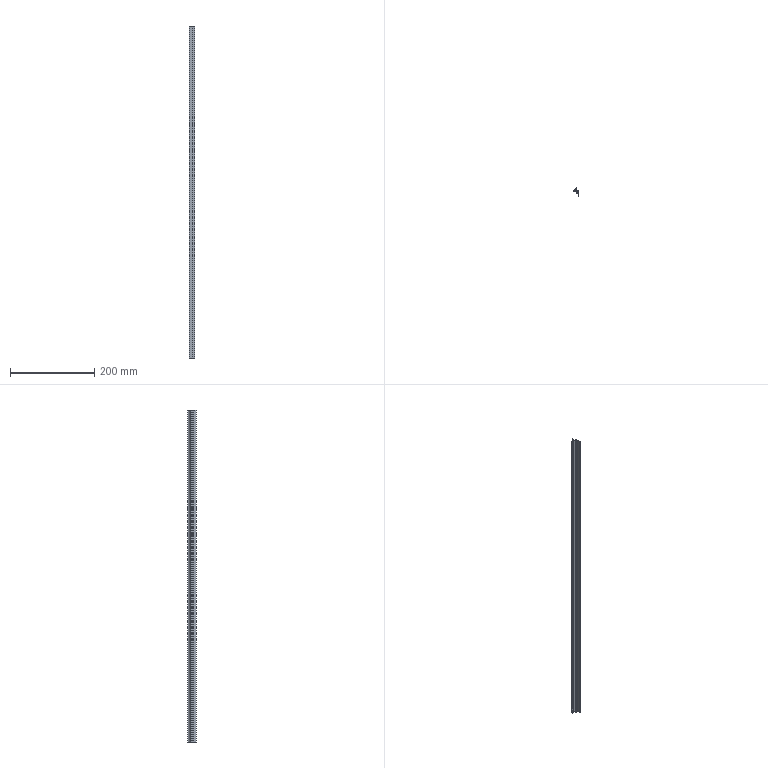Part | SolidWorks | features BaseBody 1, ICE 1, MoveFace 1 | 1 solid | 27 faces | box 14 x 20.3 x 788 mm | volume 40122 mm3 | plane 20 | cylinder 7 | commonest cylinder face diameters 0.387 x2 0.8 x2 0.4 x1 20 x1 22 x1
STEP:
#1=CARTESIAN_POINT('',(-5.304,-0.625,200.));
#2=VERTEX_POINT('',#1);
#3=CARTESIAN_POINT('',(-5.449,-0.8125,200.));
#4=VERTEX_POINT('',#3);
#5=CARTESIAN_POINT('',(-5.255,-0.8125,200.));
#6=DIRECTION('',(0.,0.,1.));
#7=DIRECTION('',(-1.,0.,0.));
#8=AXIS2_PLACEMENT_3D('',#5,#6,#7);
#9=CIRCLE('',#8,0.1937);
#10=EDGE_CURVE('',#2,#4,#9,.T.);
#11=ORIENTED_EDGE('',*,*,#10,.T.);
#12=CARTESIAN_POINT('',(-5.449,-0.8125,-588.));
#13=VERTEX_POINT('',#12);
#14=CARTESIAN_POINT('',(-5.449,-0.8125,230.));
#15=DIRECTION('',(0.,0.,-1.));
#16=VECTOR('',#15,1000.);
#17=LINE('',#14,#16);
#18=EDGE_CURVE('',#4,#13,#17,.T.);
#19=ORIENTED_EDGE('',*,*,#18,.T.);
#20=CARTESIAN_POINT('',(-5.304,-0.625,-588.));
#21=VERTEX_POINT('',#20);
#22=CARTESIAN_POINT('',(-5.255,-0.8125,-588.));
#23=DIRECTION('',(0.,0.,-1.));
#24=DIRECTION('',(1.,0.,0.));
#25=AXIS2_PLACEMENT_3D('',#22,#23,#24);
#26=CIRCLE('',#25,0.1937);
#27=EDGE_CURVE('',#13,#21,#26,.T.);
#28=ORIENTED_EDGE('',*,*,#27,.T.);
#29=CARTESIAN_POINT('',(-5.304,-0.625,230.));
#30=DIRECTION('',(0.,0.,-1.));
#31=VECTOR('',#30,1000.);
#32=LINE('',#29,#31);
#33=EDGE_CURVE('',#2,#21,#32,.T.);
#34=ORIENTED_EDGE('',*,*,#33,.F.);
#35=EDGE_LOOP('',(#11,#19,#28,#34));
#36=FACE_OUTER_BOUND('',#35,.T.);
#37=CARTESIAN_POINT('',(-5.255,-0.8125,230.));
#38=DIRECTION('',(0.,0.,-1.));
#39=DIRECTION('',(-1.,0.,0.));
#40=AXIS2_PLACEMENT_3D('',#37,#38,#39);
#41=CYLINDRICAL_SURFACE('',#40,0.1937);
#42=ADVANCED_FACE('',(#36),#41,.F.);
#43=CARTESIAN_POINT('',(5.,-1.,-588.));
#44=VERTEX_POINT('',#43);
#45=CARTESIAN_POINT('',(5.,-14.3,-588.));
#46=VERTEX_POINT('',#45);
#47=CARTESIAN_POINT('',(5.,29.623,-588.));
#48=DIRECTION('',(0.,-1.,0.));
#49=VECTOR('',#48,1000.);
#50=LINE('',#47,#49);
#51=EDGE_CURVE('',#44,#46,#50,.T.);
#52=ORIENTED_EDGE('',*,*,#51,.F.);
#53=CARTESIAN_POINT('',(5.,-1.,200.));
#54=VERTEX_POINT('',#53);
#55=CARTESIAN_POINT('',(5.,-1.,230.));
#56=DIRECTION('',(0.,0.,-1.));
#57=VECTOR('',#56,1000.);
#58=LINE('',#55,#57);
#59=EDGE_CURVE('',#54,#44,#58,.T.);
#60=ORIENTED_EDGE('',*,*,#59,.F.);
#61=CARTESIAN_POINT('',(5.,-14.3,200.));
#62=VERTEX_POINT('',#61);
#63=CARTESIAN_POINT('',(5.,-14.3,200.));
#64=DIRECTION('',(0.,1.,0.));
#65=VECTOR('',#64,1000.);
#66=LINE('',#63,#65);
#67=EDGE_CURVE('',#62,#54,#66,.T.);
#68=ORIENTED_EDGE('',*,*,#67,.F.);
#69=CARTESIAN_POINT('',(5.,-14.3,230.));
#70=DIRECTION('',(0.,0.,1.));
#71=VECTOR('',#70,1000.);
#72=LINE('',#69,#71);
#73=EDGE_CURVE('',#46,#62,#72,.T.);
#74=ORIENTED_EDGE('',*,*,#73,.F.);
#75=EDGE_LOOP('',(#52,#60,#68,#74));
#76=FACE_OUTER_BOUND('',#75,.T.);
#77=CARTESIAN_POINT('',(5.,-14.3,230.));
#78=DIRECTION('',(-1.,0.,0.));
#79=DIRECTION('',(0.,0.,1.));
#80=AXIS2_PLACEMENT_3D('',#77,#78,#79);
#81=PLANE('',#80);
#82=ADVANCED_FACE('',(#76),#81,.F.);
#83=CARTESIAN_POINT('',(-9.,-2.,-588.));
#84=VERTEX_POINT('',#83);
#85=CARTESIAN_POINT('',(-9.,-2.,200.));
#86=VERTEX_POINT('',#85);
#87=CARTESIAN_POINT('',(-9.,-2.,230.));
#88=DIRECTION('',(0.,0.,1.));
#89=VECTOR('',#88,1000.);
#90=LINE('',#87,#89);
#91=EDGE_CURVE('',#84,#86,#90,.T.);
#92=ORIENTED_EDGE('',*,*,#91,.F.);
#93=CARTESIAN_POINT('',(0.9,-2.,-588.));
#94=VERTEX_POINT('',#93);
#95=CARTESIAN_POINT('',(5.,-2.,-588.));
#96=DIRECTION('',(-1.,0.,0.));
#97=VECTOR('',#96,1000.);
#98=LINE('',#95,#97);
#99=EDGE_CURVE('',#94,#84,#98,.T.);
#100=ORIENTED_EDGE('',*,*,#99,.F.);
#101=CARTESIAN_POINT('',(0.9,-2.,200.));
#102=VERTEX_POINT('',#101);
#103=CARTESIAN_POINT('',(0.9,-2.,230.));
#104=DIRECTION('',(0.,0.,-1.));
#105=VECTOR('',#104,1000.);
#106=LINE('',#103,#105);
#107=EDGE_CURVE('',#102,#94,#106,.T.);
#108=ORIENTED_EDGE('',*,*,#107,.F.);
#109=CARTESIAN_POINT('',(5.,-2.,200.));
#110=DIRECTION('',(1.,0.,0.));
#111=VECTOR('',#110,1000.);
#112=LINE('',#109,#111);
#113=EDGE_CURVE('',#86,#102,#112,.T.);
#114=ORIENTED_EDGE('',*,*,#113,.F.);
#115=EDGE_LOOP('',(#92,#100,#108,#114));
#116=FACE_OUTER_BOUND('',#115,.T.);
#117=CARTESIAN_POINT('',(-9.,-2.,230.));
#118=DIRECTION('',(0.,1.,0.));
#119=DIRECTION('',(0.,0.,1.));
#120=AXIS2_PLACEMENT_3D('',#117,#118,#119);
#121=PLANE('',#120);
#122=ADVANCED_FACE('',(#116),#121,.F.);
#123=CARTESIAN_POINT('',(4.,-6.,200.));
#124=VERTEX_POINT('',#123);
#125=CARTESIAN_POINT('',(4.,-3.,200.));
#126=VERTEX_POINT('',#125);
#127=CARTESIAN_POINT('',(4.,29.623,200.));
#128=DIRECTION('',(0.,1.,0.));
#129=VECTOR('',#128,1000.);
#130=LINE('',#127,#129);
#131=EDGE_CURVE('',#124,#126,#130,.T.);
#132=ORIENTED_EDGE('',*,*,#131,.F.);
#133=CARTESIAN_POINT('',(1.,-6.,200.));
#134=VERTEX_POINT('',#133);
#135=CARTESIAN_POINT('',(5.,-6.,200.));
#136=DIRECTION('',(1.,0.,0.));
#137=VECTOR('',#136,1000.);
#138=LINE('',#135,#137);
#139=EDGE_CURVE('',#134,#124,#138,.T.);
#140=ORIENTED_EDGE('',*,*,#139,.F.);
#141=CARTESIAN_POINT('',(1.,-6.7,200.));
#142=VERTEX_POINT('',#141);
#143=CARTESIAN_POINT('',(1.,-6.,200.));
#144=DIRECTION('',(0.,-1.,0.));
#145=VECTOR('',#144,1000.);
#146=LINE('',#143,#145);
#147=EDGE_CURVE('',#134,#142,#146,.T.);
#148=ORIENTED_EDGE('',*,*,#147,.T.);
#149=CARTESIAN_POINT('',(-1.7,-6.7,200.));
#150=VERTEX_POINT('',#149);
#151=CARTESIAN_POINT('',(5.,-6.7,200.));
#152=DIRECTION('',(1.,0.,0.));
#153=VECTOR('',#152,1000.);
#154=LINE('',#151,#153);
#155=EDGE_CURVE('',#150,#142,#154,.T.);
#156=ORIENTED_EDGE('',*,*,#155,.F.);
#157=CARTESIAN_POINT('',(-1.7,-7.7,200.));
#158=VERTEX_POINT('',#157);
#159=CARTESIAN_POINT('',(-1.7,-6.7,200.));
#160=DIRECTION('',(0.,-1.,0.));
#161=VECTOR('',#160,1000.);
#162=LINE('',#159,#161);
#163=EDGE_CURVE('',#150,#158,#162,.T.);
#164=ORIENTED_EDGE('',*,*,#163,.T.);
#165=CARTESIAN_POINT('',(4.,-7.7,200.));
#166=VERTEX_POINT('',#165);
#167=CARTESIAN_POINT('',(5.,-7.7,200.));
#168=DIRECTION('',(-1.,0.,0.));
#169=VECTOR('',#168,1000.);
#170=LINE('',#167,#169);
#171=EDGE_CURVE('',#166,#158,#170,.T.);
#172=ORIENTED_EDGE('',*,*,#171,.F.);
#173=CARTESIAN_POINT('',(4.,-14.3,200.));
#174=VERTEX_POINT('',#173);
#175=CARTESIAN_POINT('',(4.,29.623,200.));
#176=DIRECTION('',(0.,1.,0.));
#177=VECTOR('',#176,1000.);
#178=LINE('',#175,#177);
#179=EDGE_CURVE('',#174,#166,#178,.T.);
#180=ORIENTED_EDGE('',*,*,#179,.F.);
#181=CARTESIAN_POINT('',(5.,-14.3,200.));
#182=DIRECTION('',(-1.,0.,0.));
#183=VECTOR('',#182,1000.);
#184=LINE('',#181,#183);
#185=EDGE_CURVE('',#62,#174,#184,.T.);
#186=ORIENTED_EDGE('',*,*,#185,.F.);
#187=ORIENTED_EDGE('',*,*,#67,.T.);
#188=CARTESIAN_POINT('',(-5.207,-1.,200.));
#189=VERTEX_POINT('',#188);
#190=CARTESIAN_POINT('',(5.,-1.,200.));
#191=DIRECTION('',(1.,0.,0.));
#192=VECTOR('',#191,1000.);
#193=LINE('',#190,#192);
#194=EDGE_CURVE('',#189,#54,#193,.T.);
#195=ORIENTED_EDGE('',*,*,#194,.F.);
#196=CARTESIAN_POINT('',(-5.255,-0.8125,200.));
#197=DIRECTION('',(0.,0.,1.));
#198=DIRECTION('',(-1.,0.,0.));
#199=AXIS2_PLACEMENT_3D('',#196,#197,#198);
#200=CIRCLE('',#199,0.1937);
#201=EDGE_CURVE('',#4,#189,#200,.T.);
#202=ORIENTED_EDGE('',*,*,#201,.F.);
#203=ORIENTED_EDGE('',*,*,#10,.F.);
#204=CARTESIAN_POINT('',(-1.368,3.063,200.));
#205=VERTEX_POINT('',#204);
#206=CARTESIAN_POINT('',(-10.628,9.,200.));
#207=DIRECTION('',(0.,0.,1.));
#208=DIRECTION('',(-1.,0.,0.));
#209=AXIS2_PLACEMENT_3D('',#206,#207,#208);
#210=CIRCLE('',#209,11.);
#211=EDGE_CURVE('',#2,#205,#210,.T.);
#212=ORIENTED_EDGE('',*,*,#211,.T.);
#213=CARTESIAN_POINT('',(-1.,2.955,200.));
#214=VERTEX_POINT('',#213);
#215=CARTESIAN_POINT('',(-1.2,2.955,200.));
#216=DIRECTION('',(0.,0.,1.));
#217=DIRECTION('',(-1.,0.,0.));
#218=AXIS2_PLACEMENT_3D('',#215,#216,#217);
#219=CIRCLE('',#218,0.2);
#220=EDGE_CURVE('',#214,#205,#219,.T.);
#221=ORIENTED_EDGE('',*,*,#220,.F.);
#222=CARTESIAN_POINT('',(-1.,1.5,200.));
#223=VERTEX_POINT('',#222);
#224=CARTESIAN_POINT('',(-1.,2.955,200.));
#225=DIRECTION('',(0.,1.,0.));
#226=VECTOR('',#225,1000.);
#227=LINE('',#224,#226);
#228=EDGE_CURVE('',#223,#214,#227,.T.);
#229=ORIENTED_EDGE('',*,*,#228,.F.);
#230=CARTESIAN_POINT('',(0.,1.5,200.));
#231=VERTEX_POINT('',#230);
#232=CARTESIAN_POINT('',(-1.,1.5,200.));
#233=DIRECTION('',(-1.,0.,0.));
#234=VECTOR('',#233,1000.);
#235=LINE('',#232,#234);
#236=EDGE_CURVE('',#231,#223,#235,.T.);
#237=ORIENTED_EDGE('',*,*,#236,.F.);
#238=CARTESIAN_POINT('',(0.,6.,200.));
#239=VERTEX_POINT('',#238);
#240=CARTESIAN_POINT('',(0.,1.5,200.));
#241=DIRECTION('',(0.,-1.,0.));
#242=VECTOR('',#241,1000.);
#243=LINE('',#240,#242);
#244=EDGE_CURVE('',#239,#231,#243,.T.);
#245=ORIENTED_EDGE('',*,*,#244,.F.);
#246=CARTESIAN_POINT('',(-0.8,6.,200.));
#247=VERTEX_POINT('',#246);
#248=CARTESIAN_POINT('',(0.,6.,200.));
#249=DIRECTION('',(1.,0.,0.));
#250=VECTOR('',#249,1000.);
#251=LINE('',#248,#250);
#252=EDGE_CURVE('',#247,#239,#251,.T.);
#253=ORIENTED_EDGE('',*,*,#252,.F.);
#254=CARTESIAN_POINT('',(-1.178,5.731,200.));
#255=VERTEX_POINT('',#254);
#256=CARTESIAN_POINT('',(-0.8,5.6,200.));
#257=DIRECTION('',(0.,0.,1.));
#258=DIRECTION('',(-1.,0.,0.));
#259=AXIS2_PLACEMENT_3D('',#256,#257,#258);
#260=CIRCLE('',#259,0.4);
#261=EDGE_CURVE('',#247,#255,#260,.T.);
#262=ORIENTED_EDGE('',*,*,#261,.T.);
#263=CARTESIAN_POINT('',(-8.678,-0.8077,200.));
#264=VERTEX_POINT('',#263);
#265=CARTESIAN_POINT('',(-10.628,9.,200.));
#266=DIRECTION('',(0.,0.,1.));
#267=DIRECTION('',(-1.,0.,0.));
#268=AXIS2_PLACEMENT_3D('',#265,#266,#267);
#269=CIRCLE('',#268,10.);
#270=EDGE_CURVE('',#264,#255,#269,.T.);
#271=ORIENTED_EDGE('',*,*,#270,.F.);
#272=CARTESIAN_POINT('',(-9.,-1.2,200.));
#273=VERTEX_POINT('',#272);
#274=CARTESIAN_POINT('',(-8.6,-1.2,200.));
#275=DIRECTION('',(0.,0.,1.));
#276=DIRECTION('',(-1.,0.,0.));
#277=AXIS2_PLACEMENT_3D('',#274,#275,#276);
#278=CIRCLE('',#277,0.4);
#279=EDGE_CURVE('',#264,#273,#278,.T.);
#280=ORIENTED_EDGE('',*,*,#279,.T.);
#281=CARTESIAN_POINT('',(-9.,8.,200.));
#282=DIRECTION('',(0.,-1.,0.));
#283=VECTOR('',#282,1000.);
#284=LINE('',#281,#283);
#285=EDGE_CURVE('',#273,#86,#284,.T.);
#286=ORIENTED_EDGE('',*,*,#285,.T.);
#287=ORIENTED_EDGE('',*,*,#113,.T.);
#288=CARTESIAN_POINT('',(0.9,-3.,200.));
#289=VERTEX_POINT('',#288);
#290=CARTESIAN_POINT('',(0.9,29.623,200.));
#291=DIRECTION('',(0.,1.,0.));
#292=VECTOR('',#291,1000.);
#293=LINE('',#290,#292);
#294=EDGE_CURVE('',#289,#102,#293,.T.);
#295=ORIENTED_EDGE('',*,*,#294,.F.);
#296=CARTESIAN_POINT('',(5.,-3.,200.));
#297=DIRECTION('',(-1.,0.,0.));
#298=VECTOR('',#297,1000.);
#299=LINE('',#296,#298);
#300=EDGE_CURVE('',#126,#289,#299,.T.);
#301=ORIENTED_EDGE('',*,*,#300,.F.);
#302=EDGE_LOOP('',(#132,#140,#148,#156,#164,#172,#180,#186,#187,#195,#202,#203,#212,#221,#229,#237,#245,#253,#262,#271,#280,#286,#287,#295,#301));
#303=FACE_OUTER_BOUND('',#302,.T.);
#304=CARTESIAN_POINT('',(5.,29.623,200.));
#305=DIRECTION('',(0.,0.,-1.));
#306=DIRECTION('',(-1.,0.,0.));
#307=AXIS2_PLACEMENT_3D('',#304,#305,#306);
#308=PLANE('',#307);
#309=ADVANCED_FACE('',(#303),#308,.F.);
#310=ORIENTED_EDGE('',*,*,#185,.T.);
#311=CARTESIAN_POINT('',(4.,-14.3,-588.));
#312=VERTEX_POINT('',#311);
#313=CARTESIAN_POINT('',(4.,-14.3,230.));
#314=DIRECTION('',(0.,0.,1.));
#315=VECTOR('',#314,1000.);
#316=LINE('',#313,#315);
#317=EDGE_CURVE('',#312,#174,#316,.T.);
#318=ORIENTED_EDGE('',*,*,#317,.F.);
#319=CARTESIAN_POINT('',(5.,-14.3,-588.));
#320=DIRECTION('',(-1.,0.,0.));
#321=VECTOR('',#320,1000.);
#322=LINE('',#319,#321);
#323=EDGE_CURVE('',#46,#312,#322,.T.);
#324=ORIENTED_EDGE('',*,*,#323,.F.);
#325=ORIENTED_EDGE('',*,*,#73,.T.);
#326=EDGE_LOOP('',(#310,#318,#324,#325));
#327=FACE_OUTER_BOUND('',#326,.T.);
#328=CARTESIAN_POINT('',(4.,-14.3,230.));
#329=DIRECTION('',(0.,1.,0.));
#330=DIRECTION('',(0.,0.,1.));
#331=AXIS2_PLACEMENT_3D('',#328,#329,#330);
#332=PLANE('',#331);
#333=ADVANCED_FACE('',(#327),#332,.F.);
#334=ORIENTED_EDGE('',*,*,#51,.T.);
#335=ORIENTED_EDGE('',*,*,#323,.T.);
#336=CARTESIAN_POINT('',(4.,-7.7,-588.));
#337=VERTEX_POINT('',#336);
#338=CARTESIAN_POINT('',(4.,-7.7,-588.));
#339=DIRECTION('',(0.,-1.,0.));
#340=VECTOR('',#339,1000.);
#341=LINE('',#338,#340);
#342=EDGE_CURVE('',#337,#312,#341,.T.);
#343=ORIENTED_EDGE('',*,*,#342,.F.);
#344=CARTESIAN_POINT('',(-1.7,-7.7,-588.));
#345=VERTEX_POINT('',#344);
#346=CARTESIAN_POINT('',(-1.7,-7.7,-588.));
#347=DIRECTION('',(1.,0.,0.));
#348=VECTOR('',#347,1000.);
#349=LINE('',#346,#348);
#350=EDGE_CURVE('',#345,#337,#349,.T.);
#351=ORIENTED_EDGE('',*,*,#350,.F.);
#352=CARTESIAN_POINT('',(-1.7,-6.7,-588.));
#353=VERTEX_POINT('',#352);
#354=CARTESIAN_POINT('',(-1.7,29.623,-588.));
#355=DIRECTION('',(0.,1.,0.));
#356=VECTOR('',#355,1000.);
#357=LINE('',#354,#356);
#358=EDGE_CURVE('',#345,#353,#357,.T.);
#359=ORIENTED_EDGE('',*,*,#358,.T.);
#360=CARTESIAN_POINT('',(1.,-6.7,-588.));
#361=VERTEX_POINT('',#360);
#362=CARTESIAN_POINT('',(1.,-6.7,-588.));
#363=DIRECTION('',(-1.,0.,0.));
#364=VECTOR('',#363,1000.);
#365=LINE('',#362,#364);
#366=EDGE_CURVE('',#361,#353,#365,.T.);
#367=ORIENTED_EDGE('',*,*,#366,.F.);
#368=CARTESIAN_POINT('',(1.,-6.,-588.));
#369=VERTEX_POINT('',#368);
#370=CARTESIAN_POINT('',(1.,29.623,-588.));
#371=DIRECTION('',(0.,1.,0.));
#372=VECTOR('',#371,1000.);
#373=LINE('',#370,#372);
#374=EDGE_CURVE('',#361,#369,#373,.T.);
#375=ORIENTED_EDGE('',*,*,#374,.T.);
#376=CARTESIAN_POINT('',(4.,-6.,-588.));
#377=VERTEX_POINT('',#376);
#378=CARTESIAN_POINT('',(4.,-6.,-588.));
#379=DIRECTION('',(-1.,0.,0.));
#380=VECTOR('',#379,1000.);
#381=LINE('',#378,#380);
#382=EDGE_CURVE('',#377,#369,#381,.T.);
#383=ORIENTED_EDGE('',*,*,#382,.F.);
#384=CARTESIAN_POINT('',(4.,-3.,-588.));
#385=VERTEX_POINT('',#384);
#386=CARTESIAN_POINT('',(4.,-3.,-588.));
#387=DIRECTION('',(0.,-1.,0.));
#388=VECTOR('',#387,1000.);
#389=LINE('',#386,#388);
#390=EDGE_CURVE('',#385,#377,#389,.T.);
#391=ORIENTED_EDGE('',*,*,#390,.F.);
#392=CARTESIAN_POINT('',(0.9,-3.,-588.));
#393=VERTEX_POINT('',#392);
#394=CARTESIAN_POINT('',(0.9,-3.,-588.));
#395=DIRECTION('',(1.,0.,0.));
#396=VECTOR('',#395,1000.);
#397=LINE('',#394,#396);
#398=EDGE_CURVE('',#393,#385,#397,.T.);
#399=ORIENTED_EDGE('',*,*,#398,.F.);
#400=CARTESIAN_POINT('',(0.9,-2.,-588.));
#401=DIRECTION('',(0.,-1.,0.));
#402=VECTOR('',#401,1000.);
#403=LINE('',#400,#402);
#404=EDGE_CURVE('',#94,#393,#403,.T.);
#405=ORIENTED_EDGE('',*,*,#404,.F.);
#406=ORIENTED_EDGE('',*,*,#99,.T.);
#407=CARTESIAN_POINT('',(-9.,-1.2,-588.));
#408=VERTEX_POINT('',#407);
#409=CARTESIAN_POINT('',(-9.,-1.2,-588.));
#410=DIRECTION('',(0.,-1.,0.));
#411=VECTOR('',#410,1000.);
#412=LINE('',#409,#411);
#413=EDGE_CURVE('',#408,#84,#412,.T.);
#414=ORIENTED_EDGE('',*,*,#413,.F.);
#415=CARTESIAN_POINT('',(-8.678,-0.8077,-588.));
#416=VERTEX_POINT('',#415);
#417=CARTESIAN_POINT('',(-8.6,-1.2,-588.));
#418=DIRECTION('',(0.,0.,-1.));
#419=DIRECTION('',(1.,0.,0.));
#420=AXIS2_PLACEMENT_3D('',#417,#418,#419);
#421=CIRCLE('',#420,0.4);
#422=EDGE_CURVE('',#408,#416,#421,.T.);
#423=ORIENTED_EDGE('',*,*,#422,.T.);
#424=CARTESIAN_POINT('',(-1.178,5.731,-588.));
#425=VERTEX_POINT('',#424);
#426=CARTESIAN_POINT('',(-10.628,9.,-588.));
#427=DIRECTION('',(0.,0.,-1.));
#428=DIRECTION('',(1.,0.,0.));
#429=AXIS2_PLACEMENT_3D('',#426,#427,#428);
#430=CIRCLE('',#429,10.);
#431=EDGE_CURVE('',#425,#416,#430,.T.);
#432=ORIENTED_EDGE('',*,*,#431,.F.);
#433=CARTESIAN_POINT('',(-0.8,6.,-588.));
#434=VERTEX_POINT('',#433);
#435=CARTESIAN_POINT('',(-0.8,5.6,-588.));
#436=DIRECTION('',(0.,0.,-1.));
#437=DIRECTION('',(1.,0.,0.));
#438=AXIS2_PLACEMENT_3D('',#435,#436,#437);
#439=CIRCLE('',#438,0.4);
#440=EDGE_CURVE('',#425,#434,#439,.T.);
#441=ORIENTED_EDGE('',*,*,#440,.T.);
#442=CARTESIAN_POINT('',(0.,6.,-588.));
#443=VERTEX_POINT('',#442);
#444=CARTESIAN_POINT('',(0.,6.,-588.));
#445=DIRECTION('',(-1.,0.,0.));
#446=VECTOR('',#445,1000.);
#447=LINE('',#444,#446);
#448=EDGE_CURVE('',#443,#434,#447,.T.);
#449=ORIENTED_EDGE('',*,*,#448,.F.);
#450=CARTESIAN_POINT('',(0.,1.5,-588.));
#451=VERTEX_POINT('',#450);
#452=CARTESIAN_POINT('',(0.,1.5,-588.));
#453=DIRECTION('',(0.,1.,0.));
#454=VECTOR('',#453,1000.);
#455=LINE('',#452,#454);
#456=EDGE_CURVE('',#451,#443,#455,.T.);
#457=ORIENTED_EDGE('',*,*,#456,.F.);
#458=CARTESIAN_POINT('',(-1.,1.5,-588.));
#459=VERTEX_POINT('',#458);
#460=CARTESIAN_POINT('',(-1.,1.5,-588.));
#461=DIRECTION('',(1.,0.,0.));
#462=VECTOR('',#461,1000.);
#463=LINE('',#460,#462);
#464=EDGE_CURVE('',#459,#451,#463,.T.);
#465=ORIENTED_EDGE('',*,*,#464,.F.);
#466=CARTESIAN_POINT('',(-1.,2.955,-588.));
#467=VERTEX_POINT('',#466);
#468=CARTESIAN_POINT('',(-1.,2.955,-588.));
#469=DIRECTION('',(0.,-1.,0.));
#470=VECTOR('',#469,1000.);
#471=LINE('',#468,#470);
#472=EDGE_CURVE('',#467,#459,#471,.T.);
#473=ORIENTED_EDGE('',*,*,#472,.F.);
#474=CARTESIAN_POINT('',(-1.368,3.063,-588.));
#475=VERTEX_POINT('',#474);
#476=CARTESIAN_POINT('',(-1.2,2.955,-588.));
#477=DIRECTION('',(0.,0.,-1.));
#478=DIRECTION('',(1.,0.,0.));
#479=AXIS2_PLACEMENT_3D('',#476,#477,#478);
#480=CIRCLE('',#479,0.2);
#481=EDGE_CURVE('',#475,#467,#480,.T.);
#482=ORIENTED_EDGE('',*,*,#481,.F.);
#483=CARTESIAN_POINT('',(-10.628,9.,-588.));
#484=DIRECTION('',(0.,0.,-1.));
#485=DIRECTION('',(1.,0.,0.));
#486=AXIS2_PLACEMENT_3D('',#483,#484,#485);
#487=CIRCLE('',#486,11.);
#488=EDGE_CURVE('',#475,#21,#487,.T.);
#489=ORIENTED_EDGE('',*,*,#488,.T.);
#490=ORIENTED_EDGE('',*,*,#27,.F.);
#491=CARTESIAN_POINT('',(-5.207,-1.,-588.));
#492=VERTEX_POINT('',#491);
#493=CARTESIAN_POINT('',(-5.255,-0.8125,-588.));
#494=DIRECTION('',(0.,0.,-1.));
#495=DIRECTION('',(1.,0.,0.));
#496=AXIS2_PLACEMENT_3D('',#493,#494,#495);
#497=CIRCLE('',#496,0.1937);
#498=EDGE_CURVE('',#492,#13,#497,.T.);
#499=ORIENTED_EDGE('',*,*,#498,.F.);
#500=CARTESIAN_POINT('',(5.,-1.,-588.));
#501=DIRECTION('',(-1.,0.,0.));
#502=VECTOR('',#501,1000.);
#503=LINE('',#500,#502);
#504=EDGE_CURVE('',#44,#492,#503,.T.);
#505=ORIENTED_EDGE('',*,*,#504,.F.);
#506=EDGE_LOOP('',(#334,#335,#343,#351,#359,#367,#375,#383,#391,#399,#405,#406,#414,#423,#432,#441,#449,#457,#465,#473,#482,#489,#490,#499,#505));
#507=FACE_OUTER_BOUND('',#506,.T.);
#508=CARTESIAN_POINT('',(5.,29.623,-588.));
#509=DIRECTION('',(0.,0.,1.));
#510=DIRECTION('',(1.,0.,0.));
#511=AXIS2_PLACEMENT_3D('',#508,#509,#510);
#512=PLANE('',#511);
#513=ADVANCED_FACE('',(#507),#512,.F.);
#514=ORIENTED_EDGE('',*,*,#59,.T.);
#515=ORIENTED_EDGE('',*,*,#504,.T.);
#516=CARTESIAN_POINT('',(-5.207,-1.,230.));
#517=DIRECTION('',(0.,0.,-1.));
#518=VECTOR('',#517,1000.);
#519=LINE('',#516,#518);
#520=EDGE_CURVE('',#189,#492,#519,.T.);
#521=ORIENTED_EDGE('',*,*,#520,.F.);
#522=ORIENTED_EDGE('',*,*,#194,.T.);
#523=EDGE_LOOP('',(#514,#515,#521,#522));
#524=FACE_OUTER_BOUND('',#523,.T.);
#525=CARTESIAN_POINT('',(5.,-1.,230.));
#526=DIRECTION('',(0.,-1.,0.));
#527=DIRECTION('',(0.,0.,-1.));
#528=AXIS2_PLACEMENT_3D('',#525,#526,#527);
#529=PLANE('',#528);
#530=ADVANCED_FACE('',(#524),#529,.F.);
#531=CARTESIAN_POINT('',(-9.,-1.2,230.));
#532=DIRECTION('',(0.,0.,1.));
#533=VECTOR('',#532,1000.);
#534=LINE('',#531,#533);
#535=EDGE_CURVE('',#408,#273,#534,.T.);
#536=ORIENTED_EDGE('',*,*,#535,.F.);
#537=ORIENTED_EDGE('',*,*,#413,.T.);
#538=ORIENTED_EDGE('',*,*,#91,.T.);
#539=ORIENTED_EDGE('',*,*,#285,.F.);
#540=EDGE_LOOP('',(#536,#537,#538,#539));
#541=FACE_OUTER_BOUND('',#540,.T.);
#542=CARTESIAN_POINT('',(-9.,-1.2,230.));
#543=DIRECTION('',(1.,0.,0.));
#544=DIRECTION('',(0.,0.,-1.));
#545=AXIS2_PLACEMENT_3D('',#542,#543,#544);
#546=PLANE('',#545);
#547=ADVANCED_FACE('',(#541),#546,.F.);
#548=ORIENTED_EDGE('',*,*,#294,.T.);
#549=ORIENTED_EDGE('',*,*,#107,.T.);
#550=ORIENTED_EDGE('',*,*,#404,.T.);
#551=CARTESIAN_POINT('',(0.9,-3.,230.));
#552=DIRECTION('',(0.,0.,-1.));
#553=VECTOR('',#552,1000.);
#554=LINE('',#551,#553);
#555=EDGE_CURVE('',#289,#393,#554,.T.);
#556=ORIENTED_EDGE('',*,*,#555,.F.);
#557=EDGE_LOOP('',(#548,#549,#550,#556));
#558=FACE_OUTER_BOUND('',#557,.T.);
#559=CARTESIAN_POINT('',(0.9,-2.,230.));
#560=DIRECTION('',(1.,0.,0.));
#561=DIRECTION('',(0.,0.,-1.));
#562=AXIS2_PLACEMENT_3D('',#559,#560,#561);
#563=PLANE('',#562);
#564=ADVANCED_FACE('',(#558),#563,.F.);
#565=ORIENTED_EDGE('',*,*,#300,.T.);
#566=ORIENTED_EDGE('',*,*,#555,.T.);
#567=ORIENTED_EDGE('',*,*,#398,.T.);
#568=CARTESIAN_POINT('',(4.,-3.,230.));
#569=DIRECTION('',(0.,0.,-1.));
#570=VECTOR('',#569,1000.);
#571=LINE('',#568,#570);
#572=EDGE_CURVE('',#126,#385,#571,.T.);
#573=ORIENTED_EDGE('',*,*,#572,.F.);
#574=EDGE_LOOP('',(#565,#566,#567,#573));
#575=FACE_OUTER_BOUND('',#574,.T.);
#576=CARTESIAN_POINT('',(0.9,-3.,230.));
#577=DIRECTION('',(0.,1.,0.));
#578=DIRECTION('',(0.,0.,1.));
#579=AXIS2_PLACEMENT_3D('',#576,#577,#578);
#580=PLANE('',#579);
#581=ADVANCED_FACE('',(#575),#580,.F.);
#582=ORIENTED_EDGE('',*,*,#131,.T.);
#583=ORIENTED_EDGE('',*,*,#572,.T.);
#584=ORIENTED_EDGE('',*,*,#390,.T.);
#585=CARTESIAN_POINT('',(4.,-6.,230.));
#586=DIRECTION('',(0.,0.,-1.));
#587=VECTOR('',#586,1000.);
#588=LINE('',#585,#587);
#589=EDGE_CURVE('',#124,#377,#588,.T.);
#590=ORIENTED_EDGE('',*,*,#589,.F.);
#591=EDGE_LOOP('',(#582,#583,#584,#590));
#592=FACE_OUTER_BOUND('',#591,.T.);
#593=CARTESIAN_POINT('',(4.,-3.,230.));
#594=DIRECTION('',(1.,0.,0.));
#595=DIRECTION('',(0.,0.,-1.));
#596=AXIS2_PLACEMENT_3D('',#593,#594,#595);
#597=PLANE('',#596);
#598=ADVANCED_FACE('',(#592),#597,.F.);
#599=ORIENTED_EDGE('',*,*,#139,.T.);
#600=ORIENTED_EDGE('',*,*,#589,.T.);
#601=ORIENTED_EDGE('',*,*,#382,.T.);
#602=CARTESIAN_POINT('',(1.,-6.,230.));
#603=DIRECTION('',(0.,0.,-1.));
#604=VECTOR('',#603,1000.);
#605=LINE('',#602,#604);
#606=EDGE_CURVE('',#134,#369,#605,.T.);
#607=ORIENTED_EDGE('',*,*,#606,.F.);
#608=EDGE_LOOP('',(#599,#600,#601,#607));
#609=FACE_OUTER_BOUND('',#608,.T.);
#610=CARTESIAN_POINT('',(4.,-6.,230.));
#611=DIRECTION('',(0.,-1.,0.));
#612=DIRECTION('',(0.,0.,-1.));
#613=AXIS2_PLACEMENT_3D('',#610,#611,#612);
#614=PLANE('',#613);
#615=ADVANCED_FACE('',(#609),#614,.F.);
#616=ORIENTED_EDGE('',*,*,#155,.T.);
#617=CARTESIAN_POINT('',(1.,-6.7,230.));
#618=DIRECTION('',(0.,0.,1.));
#619=VECTOR('',#618,1000.);
#620=LINE('',#617,#619);
#621=EDGE_CURVE('',#361,#142,#620,.T.);
#622=ORIENTED_EDGE('',*,*,#621,.F.);
#623=ORIENTED_EDGE('',*,*,#366,.T.);
#624=CARTESIAN_POINT('',(-1.7,-6.7,230.));
#625=DIRECTION('',(0.,0.,-1.));
#626=VECTOR('',#625,1000.);
#627=LINE('',#624,#626);
#628=EDGE_CURVE('',#150,#353,#627,.T.);
#629=ORIENTED_EDGE('',*,*,#628,.F.);
#630=EDGE_LOOP('',(#616,#622,#623,#629));
#631=FACE_OUTER_BOUND('',#630,.T.);
#632=CARTESIAN_POINT('',(1.,-6.7,230.));
#633=DIRECTION('',(0.,-1.,0.));
#634=DIRECTION('',(0.,0.,-1.));
#635=AXIS2_PLACEMENT_3D('',#632,#633,#634);
#636=PLANE('',#635);
#637=ADVANCED_FACE('',(#631),#636,.F.);
#638=ORIENTED_EDGE('',*,*,#171,.T.);
#639=CARTESIAN_POINT('',(-1.7,-7.7,230.));
#640=DIRECTION('',(0.,0.,1.));
#641=VECTOR('',#640,1000.);
#642=LINE('',#639,#641);
#643=EDGE_CURVE('',#345,#158,#642,.T.);
#644=ORIENTED_EDGE('',*,*,#643,.F.);
#645=ORIENTED_EDGE('',*,*,#350,.T.);
#646=CARTESIAN_POINT('',(4.,-7.7,230.));
#647=DIRECTION('',(0.,0.,-1.));
#648=VECTOR('',#647,1000.);
#649=LINE('',#646,#648);
#650=EDGE_CURVE('',#166,#337,#649,.T.);
#651=ORIENTED_EDGE('',*,*,#650,.F.);
#652=EDGE_LOOP('',(#638,#644,#645,#651));
#653=FACE_OUTER_BOUND('',#652,.T.);
#654=CARTESIAN_POINT('',(-1.7,-7.7,230.));
#655=DIRECTION('',(0.,1.,0.));
#656=DIRECTION('',(0.,0.,1.));
#657=AXIS2_PLACEMENT_3D('',#654,#655,#656);
#658=PLANE('',#657);
#659=ADVANCED_FACE('',(#653),#658,.F.);
#660=ORIENTED_EDGE('',*,*,#179,.T.);
#661=ORIENTED_EDGE('',*,*,#650,.T.);
#662=ORIENTED_EDGE('',*,*,#342,.T.);
#663=ORIENTED_EDGE('',*,*,#317,.T.);
#664=EDGE_LOOP('',(#660,#661,#662,#663));
#665=FACE_OUTER_BOUND('',#664,.T.);
#666=CARTESIAN_POINT('',(4.,-7.7,230.));
#667=DIRECTION('',(1.,0.,0.));
#668=DIRECTION('',(0.,0.,-1.));
#669=AXIS2_PLACEMENT_3D('',#666,#667,#668);
#670=PLANE('',#669);
#671=ADVANCED_FACE('',(#665),#670,.F.);
#672=ORIENTED_EDGE('',*,*,#18,.F.);
#673=ORIENTED_EDGE('',*,*,#201,.T.);
#674=ORIENTED_EDGE('',*,*,#520,.T.);
#675=ORIENTED_EDGE('',*,*,#498,.T.);
#676=EDGE_LOOP('',(#672,#673,#674,#675));
#677=FACE_OUTER_BOUND('',#676,.T.);
#678=CARTESIAN_POINT('',(-5.255,-0.8125,230.));
#679=DIRECTION('',(0.,0.,-1.));
#680=DIRECTION('',(-1.,0.,0.));
#681=AXIS2_PLACEMENT_3D('',#678,#679,#680);
#682=CYLINDRICAL_SURFACE('',#681,0.1937);
#683=ADVANCED_FACE('',(#677),#682,.F.);
#684=CARTESIAN_POINT('',(-1.,2.955,230.));
#685=DIRECTION('',(0.,0.,1.));
#686=VECTOR('',#685,1000.);
#687=LINE('',#684,#686);
#688=EDGE_CURVE('',#467,#214,#687,.T.);
#689=ORIENTED_EDGE('',*,*,#688,.F.);
#690=ORIENTED_EDGE('',*,*,#472,.T.);
#691=CARTESIAN_POINT('',(-1.,1.5,230.));
#692=DIRECTION('',(0.,0.,-1.));
#693=VECTOR('',#692,1000.);
#694=LINE('',#691,#693);
#695=EDGE_CURVE('',#223,#459,#694,.T.);
#696=ORIENTED_EDGE('',*,*,#695,.F.);
#697=ORIENTED_EDGE('',*,*,#228,.T.);
#698=EDGE_LOOP('',(#689,#690,#696,#697));
#699=FACE_OUTER_BOUND('',#698,.T.);
#700=CARTESIAN_POINT('',(-1.,2.955,230.));
#701=DIRECTION('',(1.,0.,0.));
#702=DIRECTION('',(0.,0.,-1.));
#703=AXIS2_PLACEMENT_3D('',#700,#701,#702);
#704=PLANE('',#703);
#705=ADVANCED_FACE('',(#699),#704,.F.);
#706=ORIENTED_EDGE('',*,*,#488,.F.);
#707=CARTESIAN_POINT('',(-1.368,3.063,230.));
#708=DIRECTION('',(0.,0.,1.));
#709=VECTOR('',#708,1000.);
#710=LINE('',#707,#709);
#711=EDGE_CURVE('',#475,#205,#710,.T.);
#712=ORIENTED_EDGE('',*,*,#711,.T.);
#713=ORIENTED_EDGE('',*,*,#211,.F.);
#714=ORIENTED_EDGE('',*,*,#33,.T.);
#715=EDGE_LOOP('',(#706,#712,#713,#714));
#716=FACE_OUTER_BOUND('',#715,.T.);
#717=CARTESIAN_POINT('',(-10.628,9.,230.));
#718=DIRECTION('',(0.,0.,-1.));
#719=DIRECTION('',(-1.,0.,0.));
#720=AXIS2_PLACEMENT_3D('',#717,#718,#719);
#721=CYLINDRICAL_SURFACE('',#720,11.);
#722=ADVANCED_FACE('',(#716),#721,.T.);
#723=CARTESIAN_POINT('',(-1.178,5.731,230.));
#724=DIRECTION('',(0.,0.,1.));
#725=VECTOR('',#724,1000.);
#726=LINE('',#723,#725);
#727=EDGE_CURVE('',#425,#255,#726,.T.);
#728=ORIENTED_EDGE('',*,*,#727,.F.);
#729=ORIENTED_EDGE('',*,*,#431,.T.);
#730=CARTESIAN_POINT('',(-8.678,-0.8077,230.));
#731=DIRECTION('',(0.,0.,-1.));
#732=VECTOR('',#731,1000.);
#733=LINE('',#730,#732);
#734=EDGE_CURVE('',#264,#416,#733,.T.);
#735=ORIENTED_EDGE('',*,*,#734,.F.);
#736=ORIENTED_EDGE('',*,*,#270,.T.);
#737=EDGE_LOOP('',(#728,#729,#735,#736));
#738=FACE_OUTER_BOUND('',#737,.T.);
#739=CARTESIAN_POINT('',(-10.628,9.,230.));
#740=DIRECTION('',(0.,0.,-1.));
#741=DIRECTION('',(-1.,0.,0.));
#742=AXIS2_PLACEMENT_3D('',#739,#740,#741);
#743=CYLINDRICAL_SURFACE('',#742,10.);
#744=ADVANCED_FACE('',(#738),#743,.F.);
#745=CARTESIAN_POINT('',(0.,1.5,230.));
#746=DIRECTION('',(0.,0.,1.));
#747=VECTOR('',#746,1000.);
#748=LINE('',#745,#747);
#749=EDGE_CURVE('',#451,#231,#748,.T.);
#750=ORIENTED_EDGE('',*,*,#749,.F.);
#751=ORIENTED_EDGE('',*,*,#456,.T.);
#752=CARTESIAN_POINT('',(0.,6.,230.));
#753=DIRECTION('',(0.,0.,-1.));
#754=VECTOR('',#753,1000.);
#755=LINE('',#752,#754);
#756=EDGE_CURVE('',#239,#443,#755,.T.);
#757=ORIENTED_EDGE('',*,*,#756,.F.);
#758=ORIENTED_EDGE('',*,*,#244,.T.);
#759=EDGE_LOOP('',(#750,#751,#757,#758));
#760=FACE_OUTER_BOUND('',#759,.T.);
#761=CARTESIAN_POINT('',(0.,1.5,230.));
#762=DIRECTION('',(-1.,0.,0.));
#763=DIRECTION('',(0.,0.,1.));
#764=AXIS2_PLACEMENT_3D('',#761,#762,#763);
#765=PLANE('',#764);
#766=ADVANCED_FACE('',(#760),#765,.F.);
#767=ORIENTED_EDGE('',*,*,#422,.F.);
#768=ORIENTED_EDGE('',*,*,#535,.T.);
#769=ORIENTED_EDGE('',*,*,#279,.F.);
#770=ORIENTED_EDGE('',*,*,#734,.T.);
#771=EDGE_LOOP('',(#767,#768,#769,#770));
#772=FACE_OUTER_BOUND('',#771,.T.);
#773=CARTESIAN_POINT('',(-8.6,-1.2,230.));
#774=DIRECTION('',(0.,0.,-1.));
#775=DIRECTION('',(-1.,0.,0.));
#776=AXIS2_PLACEMENT_3D('',#773,#774,#775);
#777=CYLINDRICAL_SURFACE('',#776,0.4);
#778=ADVANCED_FACE('',(#772),#777,.T.);
#779=ORIENTED_EDGE('',*,*,#147,.F.);
#780=ORIENTED_EDGE('',*,*,#606,.T.);
#781=ORIENTED_EDGE('',*,*,#374,.F.);
#782=ORIENTED_EDGE('',*,*,#621,.T.);
#783=EDGE_LOOP('',(#779,#780,#781,#782));
#784=FACE_OUTER_BOUND('',#783,.T.);
#785=CARTESIAN_POINT('',(1.,-6.,230.));
#786=DIRECTION('',(1.,0.,0.));
#787=DIRECTION('',(0.,0.,-1.));
#788=AXIS2_PLACEMENT_3D('',#785,#786,#787);
#789=PLANE('',#788);
#790=ADVANCED_FACE('',(#784),#789,.F.);
#791=ORIENTED_EDGE('',*,*,#163,.F.);
#792=ORIENTED_EDGE('',*,*,#628,.T.);
#793=ORIENTED_EDGE('',*,*,#358,.F.);
#794=ORIENTED_EDGE('',*,*,#643,.T.);
#795=EDGE_LOOP('',(#791,#792,#793,#794));
#796=FACE_OUTER_BOUND('',#795,.T.);
#797=CARTESIAN_POINT('',(-1.7,-6.7,230.));
#798=DIRECTION('',(1.,0.,0.));
#799=DIRECTION('',(0.,0.,-1.));
#800=AXIS2_PLACEMENT_3D('',#797,#798,#799);
#801=PLANE('',#800);
#802=ADVANCED_FACE('',(#796),#801,.F.);
#803=ORIENTED_EDGE('',*,*,#711,.F.);
#804=ORIENTED_EDGE('',*,*,#481,.T.);
#805=ORIENTED_EDGE('',*,*,#688,.T.);
#806=ORIENTED_EDGE('',*,*,#220,.T.);
#807=EDGE_LOOP('',(#803,#804,#805,#806));
#808=FACE_OUTER_BOUND('',#807,.T.);
#809=CARTESIAN_POINT('',(-1.2,2.955,230.));
#810=DIRECTION('',(0.,0.,-1.));
#811=DIRECTION('',(-1.,0.,0.));
#812=AXIS2_PLACEMENT_3D('',#809,#810,#811);
#813=CYLINDRICAL_SURFACE('',#812,0.2);
#814=ADVANCED_FACE('',(#808),#813,.F.);
#815=ORIENTED_EDGE('',*,*,#695,.T.);
#816=ORIENTED_EDGE('',*,*,#464,.T.);
#817=ORIENTED_EDGE('',*,*,#749,.T.);
#818=ORIENTED_EDGE('',*,*,#236,.T.);
#819=EDGE_LOOP('',(#815,#816,#817,#818));
#820=FACE_OUTER_BOUND('',#819,.T.);
#821=CARTESIAN_POINT('',(-1.,1.5,230.));
#822=DIRECTION('',(0.,1.,0.));
#823=DIRECTION('',(0.,0.,1.));
#824=AXIS2_PLACEMENT_3D('',#821,#822,#823);
#825=PLANE('',#824);
#826=ADVANCED_FACE('',(#820),#825,.F.);
#827=ORIENTED_EDGE('',*,*,#440,.F.);
#828=ORIENTED_EDGE('',*,*,#727,.T.);
#829=ORIENTED_EDGE('',*,*,#261,.F.);
#830=CARTESIAN_POINT('',(-0.8,6.,230.));
#831=DIRECTION('',(0.,0.,-1.));
#832=VECTOR('',#831,1000.);
#833=LINE('',#830,#832);
#834=EDGE_CURVE('',#247,#434,#833,.T.);
#835=ORIENTED_EDGE('',*,*,#834,.T.);
#836=EDGE_LOOP('',(#827,#828,#829,#835));
#837=FACE_OUTER_BOUND('',#836,.T.);
#838=CARTESIAN_POINT('',(-0.8,5.6,230.));
#839=DIRECTION('',(0.,0.,-1.));
#840=DIRECTION('',(-1.,0.,0.));
#841=AXIS2_PLACEMENT_3D('',#838,#839,#840);
#842=CYLINDRICAL_SURFACE('',#841,0.4);
#843=ADVANCED_FACE('',(#837),#842,.T.);
#844=ORIENTED_EDGE('',*,*,#756,.T.);
#845=ORIENTED_EDGE('',*,*,#448,.T.);
#846=ORIENTED_EDGE('',*,*,#834,.F.);
#847=ORIENTED_EDGE('',*,*,#252,.T.);
#848=EDGE_LOOP('',(#844,#845,#846,#847));
#849=FACE_OUTER_BOUND('',#848,.T.);
#850=CARTESIAN_POINT('',(0.,6.,230.));
#851=DIRECTION('',(0.,-1.,0.));
#852=DIRECTION('',(0.,0.,-1.));
#853=AXIS2_PLACEMENT_3D('',#850,#851,#852);
#854=PLANE('',#853);
#855=ADVANCED_FACE('',(#849),#854,.F.);
#856=CLOSED_SHELL('',(#42,#82,#122,#309,#333,#513,#530,#547,#564,#581,#598,#615,#637,#659,#671,#683,#705,#722,#744,#766,#778,#790,#802,#814,#826,#843,#855));
#857=MANIFOLD_SOLID_BREP('',#856);
#858=CARTESIAN_POINT('',(0.,0.,0.));
#859=DIRECTION('',(0.,0.,1.));
#860=DIRECTION('',(1.,0.,0.));
#861=AXIS2_PLACEMENT_3D('',#858,#859,#860);
#862=(LENGTH_UNIT()NAMED_UNIT(*)SI_UNIT(.MILLI.,.METRE.));
#863=UNCERTAINTY_MEASURE_WITH_UNIT(LENGTH_MEASURE(0.00001),#862,'','');
#864=(NAMED_UNIT(*)PLANE_ANGLE_UNIT()SI_UNIT($,.RADIAN.));
#865=(NAMED_UNIT(*)SI_UNIT($,.STERADIAN.)SOLID_ANGLE_UNIT());
#866=(GEOMETRIC_REPRESENTATION_CONTEXT(3)GLOBAL_UNCERTAINTY_ASSIGNED_CONTEXT((#863))GLOBAL_UNIT_ASSIGNED_CONTEXT((#862,#864,#865))REPRESENTATION_CONTEXT('',''));
#867=ADVANCED_BREP_SHAPE_REPRESENTATION('',(#857,#861),#866);